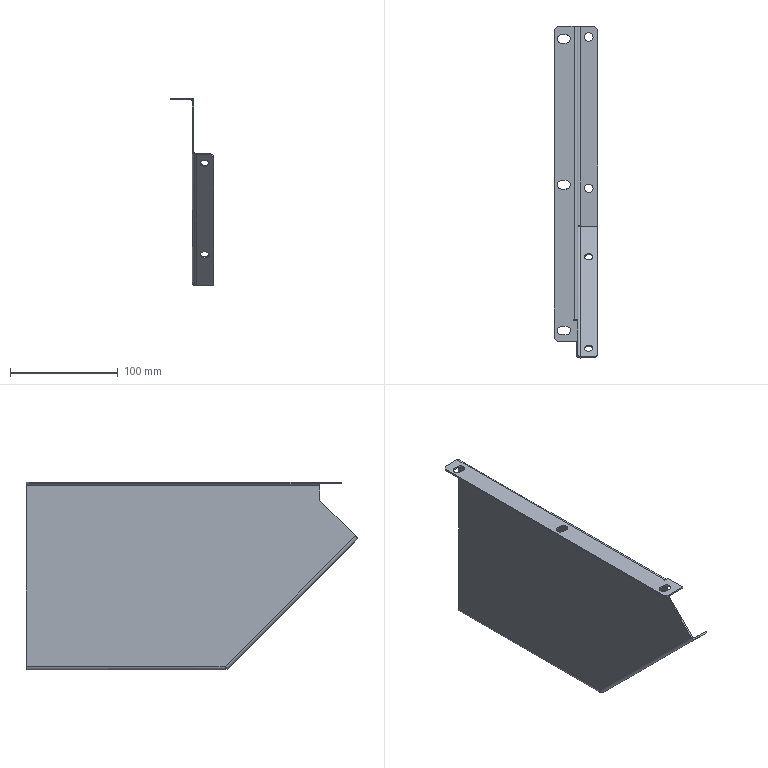Part | STEP file | SYL_0392D6J1SYL0380DJ10-1672638 | 1 solid | 68 faces | box 40.5 x 307.355 x 173.95 mm | volume 81571 mm3 | plane 40 | spline 22 | cylinder 6 | commonest cylinder face diameters 4.1 x2 7 x2 4 x1 6.9 x1